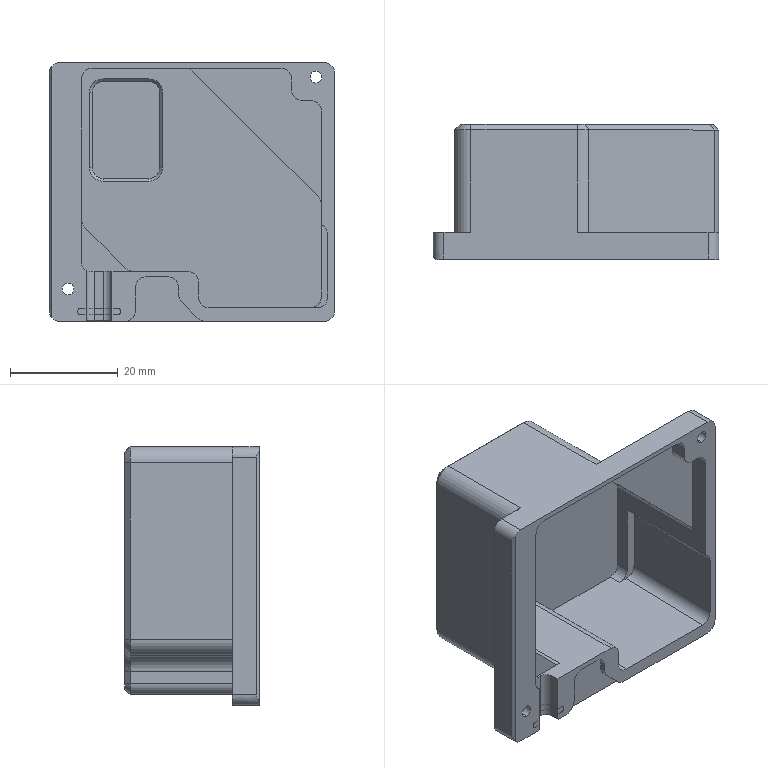NC program | NX | posted with a generic post | part box 53 x 25 x 48 mm
Lines 3425 to 5522 of 6007, first 1921 of 2086 lines:
(CAVITY_MILL_1 , TOOL : D2-6-D4-50-3T-ROUGH)
N6818 T10 M6
N6820 G54
N6822 G17 G0 G90 X25.999 Y-16.249 B0. C0. S6500 M3
N6824 G43 Z30. H10
N6826 Z3.003 B-180. C-180.
N6828 G94 G1 Z0.003 F1200.
N6830 X25.099
N6832 G3 X24.099 Y-17.25 R1.
N6834 G1 Y-18.252
N6836 X24.345 Y-18.329
N6838 X24.41 Y-18.357
N6840 X24.457 Y-18.38
N6842 X24.5 Y-18.406
N6844 X24.821 Y-18.648
N6846 X24.856 Y-18.684
N6848 X24.903 Y-18.731
N6850 X24.955 Y-18.782
N6852 X24.875 Y-19.036
N6854 X24.85 Y-19.062
N6856 X24.842 Y-19.066
N6858 X24.753 Y-18.976
N6860 X24.705 Y-18.929
N6862 X24.649 Y-18.872
N6864 X24.646 Y-18.87
N6866 X24.623 Y-18.846
N6868 X24.333 Y-18.631
N6870 X24.237 Y-18.587
N6872 X24.027 Y-18.523
N6874 X23.912 Y-18.512
N6876 Y-18.5
N6878 X14.606
N6880 X14.555 Y-18.501
N6882 X14.548 Y-18.485
N6884 X14.549 Y-18.452
N6886 X14.585 Y-18.399
N6888 X14.613 Y-18.332
N6890 X14.634 Y-18.271
N6892 X14.689 Y-17.936
N6894 X14.695 Y-16.518
N6896 X14.729 Y-16.405
N6898 X14.772 Y-16.258
N6900 X14.757 Y-16.237
N6902 X14.723 Y-16.214
N6904 X14.701 Y-16.181
N6906 X14.661 Y-16.163
N6908 X14.692 Y-16.132
N6910 X14.727 Y-16.001
N6912 X14.789 Y-16.
N6914 X15.346
N6916 X23.797 Y-15.999
N6918 X24.058 Y-15.971
N6920 G3 X24.602 Y-15.675 R0.932
N6922 G1 X24.797 Y-15.48
N6924 X24.807 Y-15.469
N6926 X24.849 Y-15.429
N6928 X24.894 Y-15.431
N6930 X24.879 Y-15.473
N6932 X24.954 Y-15.718
N6934 X24.805 Y-15.868
N6936 G2 X24.099 Y-16.248 R1.212
N6938 G1 Y-17.25
N6940 X23.199
N6942 Y-17.6
N6944 X15.589
N6946 X15.59 Y-16.9
N6948 X23.199 Y-16.899
N6950 Y-17.25
N6952 G3 X24.199 Y-18.25 R1.
N6954 G1 X25.999 Y-18.249
N6956 Z3.003
N6958 G0 Y-16.25 Z2.855
N6960 G1 Z-0.145
N6962 X25.099
N6964 G3 X24.099 Y-17.25 R1.
N6966 G1 Y-18.252
N6968 G2 X24.463 Y-18.383 R1.43
N6970 X24.841 Y-18.668 R1.431
N6972 G1 X24.903 Y-18.731
N6974 X24.955 Y-18.782
N6976 X24.875 Y-19.036
N6978 X24.842 Y-19.066
N6980 X24.753 Y-18.976
N6982 X24.613 Y-18.837
N6984 G3 X23.912 Y-18.505 R1.15
N6986 G1 Y-18.5
N6988 X23.8
N6990 X14.554 Y-18.501
N6992 X14.548 Y-18.486
N6994 X14.549 Y-18.451
N6996 X14.585 Y-18.399
N6998 X14.613 Y-18.332
N7000 X14.634 Y-18.271
N7002 X14.689 Y-17.936
N7004 X14.695 Y-16.518
N7006 X14.729 Y-16.405
N7008 X14.773 Y-16.259
N7010 X14.757 Y-16.237
N7012 X14.723 Y-16.214
N7014 X14.701 Y-16.181
N7016 X14.661 Y-16.163
N7018 X14.692 Y-16.132
N7020 X14.727 Y-16.001
N7022 X14.788 Y-16.
N7024 X23.8
N7026 G3 X24.058 Y-15.971 R1.15
N7028 X24.613 Y-15.663 R0.933
N7030 G1 X24.808 Y-15.469
N7032 X24.849 Y-15.429
N7034 X24.869 Y-15.449
N7036 X24.888 Y-15.507
N7038 X24.954 Y-15.718
N7040 X24.805 Y-15.868
N7042 G2 X24.099 Y-16.248 R1.213
N7044 G1 Y-17.25
N7046 X23.199
N7048 Y-17.6
N7050 X15.589
N7052 X15.59 Y-16.9
N7054 X23.199
N7056 Y-17.25
N7058 G3 X24.199 Y-18.25 R1.
N7060 G1 X25.999
N7062 Z2.855
N7064 G0 Y-16.25 Z2.708
N7066 G1 Z-0.293
N7068 X25.099
N7070 G3 X24.099 Y-17.25 R1.
N7072 G1 Y-18.252
N7074 G2 X24.841 Y-18.668 R1.431
N7076 G1 X24.903 Y-18.731
N7078 X24.955 Y-18.782
N7080 X24.875 Y-19.036
N7082 X24.842 Y-19.066
N7084 X24.753 Y-18.976
N7086 X24.613 Y-18.837
N7088 G3 X23.912 Y-18.505 R1.15
N7090 G1 Y-18.5
N7092 X23.8
N7094 X14.554 Y-18.501
N7096 X14.548 Y-18.486
N7098 X14.549 Y-18.451
N7100 X14.585 Y-18.399
N7102 X14.613 Y-18.332
N7104 X14.634 Y-18.271
N7106 X14.689 Y-17.936
N7108 X14.695 Y-16.518
N7110 X14.729 Y-16.405
N7112 X14.773 Y-16.259
N7114 X14.757 Y-16.237
N7116 X14.723 Y-16.214
N7118 X14.701 Y-16.181
N7120 X14.661 Y-16.163
N7122 X14.692 Y-16.132
N7124 X14.727 Y-16.001
N7126 X14.788 Y-16.
N7128 X23.8
N7130 G3 X24.058 Y-15.971 R1.15
N7132 G1 X24.188 Y-15.94
N7134 G3 X24.613 Y-15.663 R0.933
N7136 G1 X24.808 Y-15.469
N7138 X24.849 Y-15.429
N7140 X24.869 Y-15.449
N7142 X24.888 Y-15.507
N7144 X24.954 Y-15.718
N7146 X24.805 Y-15.868
N7148 G2 X24.099 Y-16.248 R1.213
N7150 G1 Y-17.25
N7152 X23.199
N7154 Y-17.6
N7156 X15.589
N7158 X15.59 Y-16.9
N7160 X23.199
N7162 Y-17.25
N7164 G3 X24.199 Y-18.25 R1.
N7166 G1 X25.999
N7168 Z2.708
N7170 G0 Y-16.25 Z2.56
N7172 G1 Z-0.44
N7174 X25.099
N7176 G3 X24.099 Y-17.25 R1.
N7178 G1 Y-18.252
N7180 G2 X24.811 Y-18.639 R1.43
N7182 G1 X24.955 Y-18.782
N7184 X24.875 Y-19.036
N7186 X24.842 Y-19.066
N7188 X24.753 Y-18.976
N7190 X24.613 Y-18.837
N7192 G3 X23.912 Y-18.505 R1.15
N7194 G1 Y-18.5
N7196 X23.8
N7198 X14.554 Y-18.501
N7200 X14.548 Y-18.486
N7202 X14.549 Y-18.452
N7204 X14.585 Y-18.399
N7206 X14.613 Y-18.332
N7208 X14.634 Y-18.271
N7210 X14.689 Y-17.936
N7212 X14.695 Y-16.518
N7214 X14.729 Y-16.405
N7216 X14.773 Y-16.259
N7218 X14.757 Y-16.237
N7220 X14.723 Y-16.214
N7222 X14.701 Y-16.181
N7224 X14.661 Y-16.163
N7226 X14.692 Y-16.132
N7228 X14.727 Y-16.001
N7230 X14.788 Y-16.
N7232 X23.8
N7234 G3 X24.058 Y-15.971 R1.15
N7236 X24.376 Y-15.858 R0.932
N7238 X24.613 Y-15.663 R0.933
N7240 G1 X24.808 Y-15.469
N7242 X24.849 Y-15.429
N7244 X24.869 Y-15.449
N7246 X24.888 Y-15.507
N7248 X24.954 Y-15.718
N7250 X24.805 Y-15.868
N7252 G2 X24.099 Y-16.248 R1.213
N7254 G1 Y-17.25
N7256 X23.199
N7258 Y-17.6
N7260 X15.589
N7262 X15.59 Y-16.9
N7264 X23.199
N7266 Y-17.25
N7268 G3 X24.199 Y-18.25 R1.
N7270 G1 X25.999
N7272 Z2.56
N7274 G0 Y-16.25 Z2.413
N7276 G1 Z-0.588
N7278 X25.099
N7280 G3 X24.099 Y-17.25 R1.
N7282 G1 Y-18.252
N7284 G2 X24.811 Y-18.639 R1.43
N7286 G1 X24.955 Y-18.782
N7288 X24.875 Y-19.036
N7290 X24.842 Y-19.066
N7292 X24.753 Y-18.976
N7294 X24.613 Y-18.837
N7296 G3 X23.912 Y-18.505 R1.15
N7298 G1 Y-18.5
N7300 X23.8
N7302 X14.554 Y-18.501
N7304 X14.548 Y-18.486
N7306 X14.549 Y-18.452
N7308 X14.585 Y-18.399
N7310 X14.613 Y-18.332
N7312 X14.634 Y-18.271
N7314 X14.689 Y-17.936
N7316 X14.695 Y-16.518
N7318 X14.729 Y-16.405
N7320 X14.773 Y-16.259
N7322 X14.757 Y-16.237
N7324 X14.723 Y-16.214
N7326 X14.701 Y-16.181
N7328 X14.661 Y-16.163
N7330 X14.692 Y-16.132
N7332 X14.727 Y-16.001
N7334 X14.788 Y-16.
N7336 X23.8
N7338 G3 X24.058 Y-15.971 R1.15
N7340 X24.613 Y-15.663 R0.933
N7342 G1 X24.849 Y-15.429
N7344 X24.869 Y-15.449
N7346 X24.888 Y-15.507
N7348 X24.954 Y-15.718
N7350 X24.805 Y-15.868
N7352 G2 X24.099 Y-16.248 R1.213
N7354 G1 Y-17.25
N7356 X23.199
N7358 Y-17.6
N7360 X15.589
N7362 X15.59 Y-16.9
N7364 X23.199
N7366 Y-17.25
N7368 G3 X24.199 Y-18.25 R1.
N7370 G1 X25.999
N7372 Z2.413
N7374 G0 Y-16.25 Z2.265
N7376 G1 Z-0.735
N7378 X25.099
N7380 G3 X24.099 Y-17.25 R1.
N7382 G1 Y-18.252
N7384 G2 X24.811 Y-18.639 R1.43
N7386 G1 X24.955 Y-18.782
N7388 X24.875 Y-19.036
N7390 X24.842 Y-19.066
N7392 X24.753 Y-18.976
N7394 X24.613 Y-18.837
N7396 G3 X23.912 Y-18.505 R1.15
N7398 G1 Y-18.5
N7400 X23.8
N7402 X14.554 Y-18.501
N7404 X14.548 Y-18.485
N7406 X14.549 Y-18.452
N7408 X14.585 Y-18.399
N7410 X14.613 Y-18.332
N7412 X14.634 Y-18.271
N7414 X14.689 Y-17.936
N7416 X14.695 Y-16.518
N7418 X14.729 Y-16.405
N7420 X14.772 Y-16.258
N7422 X14.757 Y-16.237
N7424 X14.723 Y-16.214
N7426 X14.701 Y-16.181
N7428 X14.661 Y-16.163
N7430 X14.692 Y-16.132
N7432 X14.727 Y-16.001
N7434 X14.788 Y-16.
N7436 X23.8
N7438 G3 X24.058 Y-15.971 R1.15
N7440 X24.613 Y-15.663 R0.933
N7442 G1 X24.808 Y-15.469
N7444 X24.849 Y-15.429
N7446 X24.869 Y-15.449
N7448 X24.888 Y-15.507
N7450 X24.954 Y-15.718
N7452 X24.805 Y-15.868
N7454 G2 X24.099 Y-16.248 R1.213
N7456 G1 Y-17.25
N7458 X23.199
N7460 Y-17.6
N7462 X15.589
N7464 X15.59 Y-16.9
N7466 X23.199
N7468 Y-17.25
N7470 G3 X24.199 Y-18.25 R1.
N7472 G1 X25.999
N7474 Z2.265
N7476 G0 Y-16.25 Z2.118
N7478 G1 Z-0.883
N7480 X25.099
N7482 G3 X24.099 Y-17.25 R1.
N7484 G1 Y-18.252
N7486 G2 X24.811 Y-18.639 R1.43
N7488 G1 X24.955 Y-18.782
N7490 X24.875 Y-19.036
N7492 X24.842 Y-19.066
N7494 X24.753 Y-18.976
N7496 X24.613 Y-18.837
N7498 G3 X23.912 Y-18.505 R1.15
N7500 G1 Y-18.5
N7502 X23.8
N7504 X14.554 Y-18.501
N7506 X14.548 Y-18.485
N7508 X14.549 Y-18.452
N7510 X14.585 Y-18.399
N7512 X14.613 Y-18.332
N7514 X14.634 Y-18.271
N7516 X14.689 Y-17.936
N7518 X14.695 Y-16.518
N7520 X14.729 Y-16.405
N7522 X14.773 Y-16.259
N7524 X14.757 Y-16.237
N7526 X14.723 Y-16.214
N7528 X14.701 Y-16.181
N7530 X14.661 Y-16.163
N7532 X14.692 Y-16.132
N7534 X14.727 Y-16.001
N7536 X14.788 Y-16.
N7538 X23.8
N7540 G3 X24.058 Y-15.971 R1.15
N7542 X24.613 Y-15.663 R0.933
N7544 G1 X24.808 Y-15.469
N7546 X24.849 Y-15.429
N7548 X24.869 Y-15.449
N7550 X24.888 Y-15.507
N7552 X24.954 Y-15.718
N7554 X24.805 Y-15.868
N7556 G2 X24.099 Y-16.248 R1.213
N7558 G1 Y-17.25
N7560 X23.199
N7562 Y-17.6
N7564 X15.589
N7566 X15.59 Y-16.9
N7568 X23.199
N7570 Y-17.25
N7572 G3 X24.199 Y-18.25 R1.
N7574 G1 X25.999
N7576 Z2.118
N7578 G0 Y-16.25 Z1.97
N7580 G1 Z-1.03
N7582 X25.099
N7584 G3 X24.099 Y-17.25 R1.
N7586 G1 Y-18.252
N7588 G2 X24.811 Y-18.639 R1.43
N7590 G1 X24.955 Y-18.782
N7592 X24.875 Y-19.036
N7594 X24.842 Y-19.066
N7596 X24.753 Y-18.976
N7598 X24.613 Y-18.837
N7600 G3 X23.912 Y-18.505 R1.15
N7602 G1 Y-18.5
N7604 X23.8
N7606 X14.554 Y-18.501
N7608 X14.548 Y-18.485
N7610 X14.549 Y-18.453
N7612 X14.585 Y-18.399
N7614 X14.613 Y-18.332
N7616 X14.634 Y-18.271
N7618 X14.689 Y-17.936
N7620 X14.695 Y-16.518
N7622 X14.729 Y-16.405
N7624 X14.773 Y-16.259
N7626 X14.757 Y-16.237
N7628 X14.723 Y-16.214
N7630 X14.701 Y-16.181
N7632 X14.661 Y-16.163
N7634 X14.692 Y-16.132
N7636 X14.727 Y-16.001
N7638 X14.788 Y-16.
N7640 X23.8
N7642 G3 X24.058 Y-15.971 R1.15
N7644 X24.613 Y-15.663 R0.933
N7646 G1 X24.808 Y-15.469
N7648 X24.849 Y-15.429
N7650 X24.869 Y-15.449
N7652 X24.888 Y-15.507
N7654 X24.954 Y-15.718
N7656 X24.805 Y-15.868
N7658 G2 X24.099 Y-16.248 R1.213
N7660 G1 Y-17.25
N7662 X23.199
N7664 Y-17.6
N7666 X15.589
N7668 X15.59 Y-16.9
N7670 X23.199
N7672 Y-17.25
N7674 G3 X24.199 Y-18.25 R1.
N7676 G1 X25.999
N7678 Z1.97
N7680 G0 Y-16.25 Z1.823
N7682 G1 Z-1.178
N7684 X25.099
N7686 G3 X24.099 Y-17.25 R1.
N7688 G1 Y-18.252
N7690 G2 X24.811 Y-18.639 R1.43
N7692 G1 X24.955 Y-18.782
N7694 X24.875 Y-19.036
N7696 X24.842 Y-19.066
N7698 X24.753 Y-18.976
N7700 X24.613 Y-18.837
N7702 G3 X23.912 Y-18.505 R1.15
N7704 G1 Y-18.5
N7706 X23.8
N7708 X14.554 Y-18.501
N7710 X14.548 Y-18.484
N7712 X14.549 Y-18.453
N7714 X14.585 Y-18.399
N7716 X14.613 Y-18.332
N7718 X14.634 Y-18.271
N7720 X14.689 Y-17.936
N7722 X14.695 Y-16.518
N7724 X14.729 Y-16.405
N7726 X14.773 Y-16.259
N7728 X14.757 Y-16.237
N7730 X14.723 Y-16.214
N7732 X14.701 Y-16.181
N7734 X14.661 Y-16.163
N7736 X14.692 Y-16.132
N7738 X14.727 Y-16.001
N7740 X14.735 Y-16.
N7742 X14.788
N7744 X23.8
N7746 G3 X24.058 Y-15.971 R1.15
N7748 X24.613 Y-15.663 R0.933
N7750 G1 X24.849 Y-15.429
N7752 X24.869 Y-15.449
N7754 X24.888 Y-15.507
N7756 X24.954 Y-15.718
N7758 X24.805 Y-15.868
N7760 G2 X24.099 Y-16.248 R1.213
N7762 G1 Y-17.25
N7764 X23.199
N7766 Y-17.6
N7768 X15.589
N7770 X15.59 Y-16.9
N7772 X23.199
N7774 Y-17.25
N7776 G3 X24.199 Y-18.25 R1.
N7778 G1 X25.999
N7780 Z1.823
N7782 G0 Y-16.25 Z1.675
N7784 G1 Z-1.325
N7786 X25.099
N7788 G3 X24.099 Y-17.25 R1.
N7790 G1 Y-18.252
N7792 G2 X24.811 Y-18.639 R1.43
N7794 G1 X24.955 Y-18.782
N7796 X24.875 Y-19.036
N7798 X24.842 Y-19.066
N7800 X24.753 Y-18.976
N7802 X24.613 Y-18.837
N7804 G3 X23.912 Y-18.505 R1.15
N7806 G1 Y-18.5
N7808 X23.8
N7810 X14.554 Y-18.501
N7812 X14.548 Y-18.484
N7814 X14.549 Y-18.453
N7816 X14.585 Y-18.399
N7818 X14.613 Y-18.332
N7820 X14.634 Y-18.271
N7822 X14.689 Y-17.936
N7824 X14.695 Y-16.518
N7826 X14.729 Y-16.405
N7828 X14.773 Y-16.259
N7830 X14.757 Y-16.237
N7832 X14.723 Y-16.214
N7834 X14.701 Y-16.181
N7836 X14.661 Y-16.163
N7838 X14.692 Y-16.132
N7840 X14.727 Y-16.001
N7842 X14.788 Y-16.
N7844 X23.8
N7846 G3 X24.058 Y-15.971 R1.15
N7848 G1 X24.236 Y-15.923
N7850 G3 X24.613 Y-15.663 R0.933
N7852 G1 X24.808 Y-15.469
N7854 X24.849 Y-15.429
N7856 X24.869 Y-15.449
N7858 X24.888 Y-15.507
N7860 X24.954 Y-15.718
N7862 X24.805 Y-15.868
N7864 G2 X24.099 Y-16.248 R1.213
N7866 G1 Y-17.25
N7868 X23.199
N7870 Y-17.6
N7872 X15.589
N7874 X15.59 Y-16.9
N7876 X23.199
N7878 Y-17.25
N7880 G3 X24.199 Y-18.25 R1.
N7882 G1 X25.999
N7884 Z1.675
N7886 G0 Y-16.25 Z1.528
N7888 G1 Z-1.473
N7890 X25.099
N7892 G3 X24.099 Y-17.25 R1.
N7894 G1 Y-18.252
N7896 G2 X24.834 Y-18.661 R1.43
N7898 G1 X24.955 Y-18.782
N7900 X24.876 Y-19.035
N7902 X24.843 Y-19.065
N7904 X24.805 Y-19.027
N7906 X24.753 Y-18.976
N7908 X24.613 Y-18.837
N7910 G3 X23.912 Y-18.505 R1.15
N7912 G1 Y-18.5
N7914 X23.797
N7916 X14.554 Y-18.501
N7918 X14.548 Y-18.484
N7920 X14.549 Y-18.454
N7922 X14.585 Y-18.399
N7924 X14.613 Y-18.332
N7926 X14.634 Y-18.271
N7928 X14.689 Y-17.936
N7930 X14.695 Y-16.518
N7932 X14.729 Y-16.405
N7934 X14.773 Y-16.259
N7936 X14.757 Y-16.237
N7938 X14.723 Y-16.214
N7940 X14.701 Y-16.181
N7942 X14.661 Y-16.163
N7944 X14.692 Y-16.132
N7946 X14.726 Y-16.004
N7948 X14.833 Y-16.
N7950 X23.8
N7952 G3 X24.058 Y-15.971 R1.15
N7954 X24.613 Y-15.663 R0.933
N7956 G1 X24.808 Y-15.469
N7958 X24.849 Y-15.429
N7960 X24.869 Y-15.449
N7962 X24.888 Y-15.507
N7964 X24.954 Y-15.718
N7966 X24.805 Y-15.868
N7968 G2 X24.099 Y-16.248 R1.213
N7970 G1 Y-17.25
N7972 X23.199
N7974 Y-17.6
N7976 X15.589
N7978 X15.59 Y-16.9
N7980 X23.199
N7982 Y-17.25
N7984 G3 X24.199 Y-18.25 R1.
N7986 G1 X25.999
N7988 Z1.528
N7990 G0 Y-16.25 Z1.38
N7992 G1 Z-1.62
N7994 X25.099
N7996 G3 X24.099 Y-17.25 R1.
N7998 G1 Y-18.238
N8000 G2 X24.963 Y-18.758 R1.488
N8002 G1 X24.941 Y-18.82
N8004 X24.879 Y-19.026
N8006 X24.87 Y-19.045
N8008 X24.85 Y-19.062
N8010 X24.807 Y-19.016
N8012 G3 X23.8 Y-18.489 R1.208
N8014 G1 X14.606
N8016 X14.549
N8018 X14.548 Y-18.484
N8020 Y-18.454
N8022 X14.585 Y-18.399
N8024 X14.613 Y-18.332
N8026 X14.634 Y-18.271
N8028 X14.689 Y-17.936
N8030 X14.695 Y-16.518
N8032 X14.729 Y-16.405
N8034 X14.773 Y-16.259
N8036 X14.757 Y-16.237
N8038 X14.723 Y-16.214
N8040 X14.701 Y-16.181
N8042 X14.661 Y-16.163
N8044 X14.692 Y-16.132
N8046 X14.724 Y-16.013
N8048 X15.59 Y-16.011
N8050 X23.88
N8052 G3 X24.331 Y-15.893 R0.924
N8054 X24.818 Y-15.473 R1.602
N8056 G1 X24.855 Y-15.433
N8058 X24.861 Y-15.439
N8060 X24.879 Y-15.473
N8062 X24.94 Y-15.68
N8064 X24.962 Y-15.738
N8066 G2 X24.468 Y-16.138 R1.882
N8068 X24.099 Y-16.271 R1.204
N8070 G1 Y-17.25
N8072 X23.199
N8074 Y-17.589
N8076 X15.589
N8078 X15.59 Y-16.911
N8080 X23.199
N8082 Y-17.25
N8084 G3 X24.199 Y-18.25 R1.
N8086 G1 X25.999
N8088 Z1.38
N8090 G0 Y-16.25 Z1.233
N8092 G1 Z-1.768
N8094 X25.099
N8096 G3 X24.099 Y-17.25 R1.
N8098 G1 Y-18.211
N8100 G2 X24.97 Y-18.739 R1.495
N8102 G1 X24.941 Y-18.82
N8104 X24.879 Y-19.026
N8106 X24.864 Y-19.052
N8108 X24.821 Y-19.009
N8110 G3 X23.8 Y-18.462 R1.215
N8112 G1 X14.621
N8114 X14.547
N8116 X14.558 Y-18.434
N8118 X14.585 Y-18.399
N8120 X14.613 Y-18.332
N8122 X14.634 Y-18.271
N8124 X14.689 Y-17.936
N8126 X14.695 Y-16.518
N8128 X14.729 Y-16.405
N8130 X14.772 Y-16.258
N8132 X14.757 Y-16.237
N8134 X14.723 Y-16.214
N8136 X14.701 Y-16.181
N8138 X14.661 Y-16.163
N8140 X14.692 Y-16.132
N8142 X14.717 Y-16.039
N8144 X15.59 Y-16.038
N8146 X23.8
N8148 G3 X24.839 Y-15.473 R1.25
N8150 G1 X24.866 Y-15.444
N8152 X24.888 Y-15.507
N8154 X24.94 Y-15.68
N8156 X24.971 Y-15.765
N8158 G2 X24.099 Y-16.287 R1.53
N8160 G1 Y-17.25
N8162 X23.199
N8164 Y-17.562
N8166 X15.589
N8168 X15.59 Y-16.938
N8170 X23.199
N8172 Y-17.25
N8174 G3 X24.199 Y-18.25 R1.
N8176 G1 X25.999
N8178 Z1.233
N8180 G0 Y-16.25 Z1.085
N8182 G1 Z-1.915
N8184 X25.099
N8186 G3 X24.099 Y-17.25 R1.
N8188 G1 Y-18.162
N8190 G2 X24.891 Y-18.625 R1.379
N8192 G1 X24.976 Y-18.723
N8194 X24.941 Y-18.82
N8196 X24.877 Y-19.032
N8198 X24.829 Y-18.982
N8200 X24.678 Y-18.807
N8202 G3 X23.8 Y-18.417 R1.099
N8204 G1 X14.642
N8206 X14.569 Y-18.42
N8208 X14.585 Y-18.399
N8210 X14.613 Y-18.332
N8212 X14.634 Y-18.271
N8214 X14.689 Y-17.936
N8216 X14.695 Y-16.518
N8218 X14.729 Y-16.405
N8220 X14.771 Y-16.258
N8222 X14.757 Y-16.237
N8224 X14.723 Y-16.214
N8226 X14.701 Y-16.181
N8228 X14.661 Y-16.163
N8230 X14.692 Y-16.132
N8232 X14.705 Y-16.082
N8234 X15.59 Y-16.083
N8236 X23.8
N8238 G3 X24.84 Y-15.512 R1.298
N8240 G1 X24.878 Y-15.469
N8242 X24.94 Y-15.68
N8244 X24.981 Y-15.79
N8246 G2 X24.099 Y-16.327 R1.578
N8248 G1 Y-17.25
N8250 X23.199
N8252 Y-17.517
N8254 X15.589
N8256 X15.59 Y-16.983
N8258 X23.199
N8260 Y-17.25
N8262 G3 X24.199 Y-18.25 R1.
N8264 G1 X25.999
N8266 Z1.085
N8268 G0 Y-16.25 Z0.938
N8270 G1 Z-2.063
N8272 X25.099
N8274 G3 X24.099 Y-17.25 R1.
N8276 G1 Y-18.092
N8278 G2 X24.781 Y-18.458 R1.238
N8280 G1 X24.992 Y-18.68
N8282 X24.941 Y-18.82
N8284 X24.891 Y-18.984
N8286 X24.85 Y-18.937
N8288 X24.578 Y-18.651
N8290 G3 X23.884 Y-18.353 R0.958
N8292 G1 X14.603 Y-18.355
N8294 X14.634 Y-18.271
N8296 X14.689 Y-17.936
N8298 X14.695 Y-16.518
N8300 X14.729 Y-16.405
N8302 X14.773 Y-16.259
N8304 X14.757 Y-16.237
N8306 X14.723 Y-16.214
N8308 X14.701 Y-16.181
N8310 X14.69 Y-16.147
N8312 X14.75
N8314 X23.854
N8316 G3 X24.559 Y-15.857 R1.
N8318 G1 X24.843 Y-15.575
N8320 X24.891 Y-15.516
N8322 X24.94 Y-15.68
N8324 X24.992 Y-15.821
N8326 X24.756 Y-16.056
N8328 G2 X24.099 Y-16.403 R1.28
N8330 G1 Y-17.25
N8332 X23.199
N8334 Y-17.453
N8336 X15.589
N8338 X15.59 Y-17.047
N8340 X23.199
N8342 Y-17.25
N8344 G3 X24.199 Y-18.25 R1.
N8346 G1 X25.999
N8348 Z0.938
N8350 G0 Y-16.25 Z0.79
N8352 G1 Z-2.21
N8354 X25.099
N8356 G3 X24.099 Y-17.25 R1.
N8358 G1 Y-18.007
N8360 G2 X24.814 Y-18.402 R1.293
N8362 G1 X24.945 Y-18.542
N8364 X24.999 Y-18.6
N8366 Y-18.659
N8368 X24.941 Y-18.82
N8370 X24.906 Y-18.935
N8372 X24.817 Y-18.822
N8374 X24.766 Y-18.756
N8376 X24.74 Y-18.735
N8378 X24.609 Y-18.592
N8380 G3 X23.864 Y-18.266 R1.013
N8382 G1 X14.698
N8384 X14.635 Y-18.268
N8386 X14.689 Y-17.936
N8388 X14.695 Y-16.518
N8390 X14.729 Y-16.405
N8392 X14.773 Y-16.259
N8394 X14.757 Y-16.237
N8396 X14.749 Y-16.234
N8398 X15.59
N8400 X23.8
N8402 G3 X24.852 Y-15.634 R1.342
N8404 G1 X24.906 Y-15.566
N8406 X24.94 Y-15.68
N8408 X24.999 Y-15.841
N8410 Y-15.907
N8412 G2 X24.099 Y-16.474 R1.622
N8414 G1 Y-17.25
N8416 X23.199
N8418 Y-17.366
N8420 X15.589
N8422 X15.59 Y-17.134
N8424 X23.199
N8426 Y-17.25
N8428 G3 X24.199 Y-18.25 R1.
N8430 G1 X25.999
N8432 Z0.79
N8434 G0 Y-16.239 Z0.643
N8436 G1 Z-2.358
N8438 X25.099
N8440 G3 X24.099 Y-17.239 R1.
N8442 G1 Y-17.889
N8444 G2 X24.909 Y-18.392 R1.276
N8446 G1 X24.999 Y-18.515
N8448 Y-18.659
N8450 X24.922 Y-18.881
N8452 X24.683 Y-18.558
N8454 G3 X23.88 Y-18.149 R0.996
N8456 G1 X14.726
N8458 X14.654 Y-18.153
N8460 X14.689 Y-17.936
N8462 X14.695 Y-16.518
N8464 X14.729 Y-16.405
N8466 X14.745 Y-16.351
N8468 X23.8
N8470 G3 X24.865 Y-15.699 R1.317
N8472 G1 X24.924 Y-15.625
N8474 X24.94 Y-15.68
N8476 X24.999 Y-15.841
N8478 Y-16.002
N8480 G2 X24.099 Y-16.589 R1.597
N8482 G1 Y-17.239
N8484 G3 X25.099 Y-18.239 R1.
N8486 G1 X25.999
N8488 Z0.643
N8490 G0 Y-16.238 Z0.495
N8492 G1 Z-2.505
N8494 X25.099
N8496 G3 X24.099 Y-17.238 R1.
N8498 G1 Y-17.722
N8500 G2 X24.62 Y-17.956 R1.019
N8502 X24.999 Y-18.363 R2.447
N8504 G1 Y-18.659
N8506 X24.947 Y-18.803
N8508 G3 X24.438 Y-18.169 R2.167
N8510 X23.959 Y-17.992 R0.739
N8512 G1 X14.746
N8514 X14.679 Y-17.996
N8516 X14.689 Y-17.936
N8518 X14.696 Y-16.515
N8520 X14.75 Y-16.508
N8522 X23.8
N8524 G3 X24.894 Y-15.776 R1.205
N8526 G1 X24.946 Y-15.696
N8528 X24.999 Y-15.841
N8530 Y-16.159
N8532 G2 X24.099 Y-16.754 R1.485
N8534 G1 Y-17.238
N8536 G3 X25.099 Y-18.238 R1.
N8538 G1 X25.999
N8540 Z0.495
N8542 G0 Y-17.384 Z0.348
N8544 G1 Z-2.653
N8546 G3 X24.999 Y-18.384 R1.
N8548 G1 Y-18.659
N8550 X24.977 Y-18.722
N8552 X24.692 Y-18.19
N8554 G3 X23.979 Y-17.764 R0.809
N8556 G1 X14.75
N8558 X14.689 Y-17.758
N8560 X14.69 Y-16.741
N8562 X14.75 Y-16.736
N8564 X23.8
N8566 G3 X24.948 Y-15.866 R1.325
N8568 G1 X24.985 Y-15.803
N8570 X24.999 Y-15.841
N8572 Y-16.36
N8574 G2 X24.099 Y-16.97 R1.605
N8576 G1 Y-17.49
N8578 G2 X24.939 Y-18.058 R1.089
N8580 G1 X24.999 Y-18.171
N8582 Y-18.384
N8584 G3 X25.999 Y-19.384 R1.
N8586 G1 X26.15
N8588 Z0.348
N8590 G0 X12.649 Y-17.258 Z0.2
N8592 G1 Z-2.8
N8594 X14.689 Y-17.259
N8596 Y-17.217
N8598 X14.75 Y-17.208
N8600 X23.8
N8602 X23.797 Y-17.292
N8604 X14.75
N8606 X14.689 Y-17.3
N8608 Y-17.259
N8610 Z0.2
N8612 G0 Z0.348
N8614 X26.147 Y-15.417
N8616 Z0.2
N8618 G1 Z-2.8
N8620 G3 X24.999 Y-15.967 R1.
N8622 G1 X24.982 Y-16.001
N8624 G2 X23.992 Y-17.298 R2.123
N8626 X24.985 Y-18.496 R1.734
N8628 G1 X24.999 Y-18.535
N8630 G3 X26.15 Y-19.184 R1.
N8632 G1 Z0.2
N8634 G0 Y-15.517 Z0.083
N8636 G1 Z-2.917
N8638 G3 X24.999 Y-16.266 R1.
N8640 G1 X24.979 Y-16.35
N8642 Y-18.15
N8644 X24.999 Y-18.231
N8646 G3 X26.15 Y-18.969 R1.
N8648 G1 Z0.083
N8650 G0 Z30.
(PLANAR_MILL_9 , TOOL : D2-6-D4-50-3T-ROUGH)
N8652 X10.25 Y-18.5 S4500
N8654 Z1.529
N8656 G1 Z-0.471 F300.
N8658 G3 X11.25 Y-19.5 R1.
N8660 G1 X13.25
N8662 G3 X13.75 Y-19. R0.5
N8664 G1 Y-17.
N8666 G3 X12.75 Y-16. R1.
N8668 G1 Z1.529
N8670 G0 X10.25 Y-18.5 Z1.057
N8672 G1 Z-0.943
N8674 G3 X11.25 Y-19.5 R1.
N8676 G1 X13.25
N8678 G3 X13.75 Y-19. R0.5
N8680 G1 Y-17.
N8682 G3 X12.75 Y-16. R1.
N8684 G1 Z1.057
N8686 G0 X10.25 Y-18.5 Z0.586
N8688 G1 Z-1.414
N8690 G3 X11.25 Y-19.5 R1.
N8692 G1 X13.25
N8694 G3 X13.75 Y-19. R0.5
N8696 G1 Y-17.
N8698 G3 X12.75 Y-16. R1.
N8700 G1 Z0.586
N8702 G0 X10.25 Y-18.5 Z0.114
N8704 G1 Z-1.886
N8706 G3 X11.25 Y-19.5 R1.
N8708 G1 X13.25
N8710 G3 X13.75 Y-19. R0.5
N8712 G1 Y-17.
N8714 G3 X12.75 Y-16. R1.
N8716 G1 Z0.114
N8718 G0 X10.25 Y-18.5 Z-0.357
N8720 G1 Z-2.357
N8722 G3 X11.25 Y-19.5 R1.
N8724 G1 X13.25
N8726 G3 X13.75 Y-19. R0.5
N8728 G1 Y-17.
N8730 G3 X12.75 Y-16. R1.
N8732 G1 Z-0.357
N8734 G0 X10.25 Y-18.5 Z-0.829
N8736 G1 Z-2.829
N8738 G3 X11.25 Y-19.5 R1.
N8740 G1 X13.25
N8742 G3 X13.75 Y-19. R0.5
N8744 G1 Y-17.
N8746 G3 X12.75 Y-16. R1.
N8748 G1 Z-0.829
N8750 G0 X10.25 Y-18.5 Z-1.3
N8752 G1 Z-3.3
N8754 G3 X11.25 Y-19.5 R1.
N8756 G1 X13.25
N8758 G3 X13.75 Y-19. R0.5
N8760 G1 Y-17.
N8762 G3 X12.75 Y-16. R1.
N8764 G1 Z-1.3
N8766 G0 Z30.
N8768 M5
(AREA_MILL , TOOL : 球刀R0.75-3-D4-50)
N8770 T11 M6
N8772 G54
N8774 G17 G0 G90 X13.863 Y-18.9 B0. C0. S6500 M3
N8776 G43 Z30. H11
N8778 Z2.815 B-180. C-180.
N8780 G94 G1 Z0. F2000.
N8782 X13.964 Z-0.375
N8784 X14.238 Z-0.649
N8786 X14.613 Z-0.75
N8788 X23.799
N8790 X24.088 Y-18.97
N8792 X24.346 Y-19.118
N8794 X24.344 Y-19.133 Z-0.799
N8796 X24.087 Y-18.957
N8798 X23.8 Y-18.9
N8800 X14.608
N8802 X14.607 Z-0.849
N8804 X23.8
N8806 X24.087 Y-18.957
N8808 X24.33 Y-19.12
N8810 X24.349 Y-19.139
N8812 X24.355 Y-19.144 Z-0.898
N8814 X24.33 Y-19.12
N8816 X24.087 Y-18.957
N8818 X23.8 Y-18.9
N8820 X14.607
N8822 Z-0.947
N8824 X23.8
N8826 X24.087 Y-18.957
N8828 X24.33 Y-19.12
N8830 X24.36 Y-19.15
N8832 X24.366 Y-19.155 Z-0.997
N8834 X24.33 Y-19.12
N8836 X24.087 Y-18.957
N8838 X23.8 Y-18.9
N8840 X14.607
N8842 Z-1.046
N8844 X23.8
N8846 X24.087 Y-18.957
N8848 X24.33 Y-19.12
N8850 X24.371 Y-19.16
N8852 X24.377 Y-19.166 Z-1.096
N8854 X24.33 Y-19.12
N8856 X24.087 Y-18.957
N8858 X23.8 Y-18.9
N8860 X14.606
N8862 Z-1.145
N8864 X23.8
N8866 X24.087 Y-18.957
N8868 X24.33 Y-19.12
N8870 X24.382 Y-19.171
N8872 X24.385 Y-19.174 Z-1.195
N8874 X24.33 Y-19.12
N8876 X24.087 Y-18.957
N8878 X23.8 Y-18.9
N8880 X14.606
N8882 Z-1.244
N8884 X23.8
N8886 X24.087 Y-18.957
N8888 X24.33 Y-19.12
N8890 X24.391 Y-19.18
N8892 X24.396 Y-19.185 Z-1.294
N8894 X24.33 Y-19.12
N8896 X24.087 Y-18.957
N8898 X23.8 Y-18.9
N8900 X14.606
N8902 X14.605 Z-1.343
N8904 X23.8
N8906 X24.087 Y-18.957
N8908 X24.33 Y-19.12
N8910 X24.402 Y-19.191
N8912 X24.407 Y-19.197 Z-1.392
N8914 X24.33 Y-19.12
N8916 X24.087 Y-18.957
N8918 X23.8 Y-18.9
N8920 X14.605
N8922 Z-1.442
N8924 X23.8
N8926 X24.087 Y-18.957
N8928 X24.33 Y-19.12
N8930 X24.413 Y-19.202
N8932 X24.418 Y-19.208 Z-1.491
N8934 X24.33 Y-19.12
N8936 X24.087 Y-18.957
N8938 X23.8 Y-18.9
N8940 X14.605
N8942 Z-1.541
N8944 X23.8
N8946 X24.087 Y-18.957
N8948 X24.33 Y-19.12
N8950 X24.427 Y-19.216
N8952 X24.432 Y-19.222 Z-1.59
N8954 X24.33 Y-19.12
N8956 X24.087 Y-18.957
N8958 X23.8 Y-18.9
N8960 X14.604
N8962 Z-1.64
N8964 X23.8
N8966 X24.087 Y-18.957
N8968 X24.33 Y-19.12
N8970 X24.438 Y-19.227
N8972 X24.443 Y-19.232 Z-1.689
N8974 X24.33 Y-19.12
N8976 X24.087 Y-18.957
N8978 X23.8 Y-18.9
N8980 X14.604
N8982 Z-1.738
N8984 X23.8
N8986 X24.087 Y-18.957
N8988 X24.33 Y-19.12
N8990 X24.448 Y-19.238
N8992 X24.454 Y-19.243 Z-1.788
N8994 X24.33 Y-19.12
N8996 X24.087 Y-18.957
N8998 X23.8 Y-18.9
N9000 X14.604
N9002 X14.603 Z-1.837
N9004 X23.8
N9006 X24.087 Y-18.957
N9008 X24.33 Y-19.12
N9010 X24.457 Y-19.246
N9012 X24.462 Y-19.252 Z-1.887
N9014 X24.33 Y-19.12
N9016 X24.087 Y-18.957
N9018 X23.8 Y-18.9
N9020 X14.603
N9022 Z-1.936
N9024 X23.8
N9026 X24.087 Y-18.957
N9028 X24.33 Y-19.12
N9030 X24.468 Y-19.257
N9032 X24.473 Y-19.263 Z-1.986
N9034 X24.33 Y-19.12
N9036 X24.087 Y-18.957
N9038 X23.8 Y-18.9
N9040 X14.603
N9042 Z-2.035
N9044 X23.8
N9046 X24.087 Y-18.957
N9048 X24.33 Y-19.12
N9050 X24.482 Y-19.271
N9052 X24.487 Y-19.277 Z-2.085
N9054 X24.33 Y-19.12
N9056 X24.087 Y-18.957
N9058 X23.8 Y-18.9
N9060 X14.602
N9062 Z-2.134
N9064 X23.8
N9066 X24.087 Y-18.957
N9068 X24.33 Y-19.12
N9070 X24.492 Y-19.282
N9072 X24.495 Y-19.285 Z-2.183
N9074 X24.33 Y-19.12
N9076 X24.123 Y-18.973
N9078 X23.878 Y-18.904
N9080 X23.535 Y-18.9
N9082 X14.602
N9084 X14.601 Z-2.233
N9086 X23.793
N9088 X24.088 Y-18.947
N9090 X24.334 Y-19.116
N9092 X24.517 Y-19.28
N9094 X24.526 Y-19.282 Z-2.282
N9096 X24.339 Y-19.111
N9098 X24.095 Y-18.94
N9100 X23.8 Y-18.895
N9102 X14.606
N9104 X14.608 Y-18.888 Z-2.332
N9106 X23.8
N9108 X24.098 Y-18.933
N9110 X24.344 Y-19.106
N9112 X24.535 Y-19.285
N9114 X24.536 Y-19.289 Z-2.381
N9116 X24.461 Y-19.215
N9118 X24.174 Y-18.962
N9120 X23.8 Y-18.878
N9122 X14.617
N9124 X14.629 Y-18.864 Z-2.431
N9126 X23.8
N9128 X23.87 Y-18.846
N9130 X24.133 Y-18.931
N9132 X24.354 Y-19.096
N9134 X24.554 Y-19.293
N9136 X24.561 Y-19.303 Z-2.48
N9138 X24.345 Y-19.066
N9140 X24.063 Y-18.882
N9142 X23.87 Y-18.821
N9144 X23.8 Y-18.846
N9146 X14.643
N9148 X14.654 Y-18.824 Z-2.529
N9150 X23.8
N9152 X23.87 Y-18.796
N9154 X24.101 Y-18.872
N9156 X24.21 Y-18.946
N9158 X24.405 Y-19.113
N9160 X24.572 Y-19.309
N9162 X24.576 Y-19.303 Z-2.579
N9164 X24.424 Y-19.118
N9166 X24.091 Y-18.836
N9168 X23.87 Y-18.771
N9170 X23.8 Y-18.797
N9172 X14.672
N9174 X14.69 Y-18.766 Z-2.628
N9176 X23.803 Y-18.765
N9178 X23.985 Y-18.761
N9180 X24.148 Y-18.841
N9182 X24.313 Y-18.979
N9184 X24.474 Y-19.136
N9186 X24.575 Y-19.275
N9188 X24.57 Y-19.241 Z-2.678
N9190 X24.471 Y-19.118
N9192 X24.144 Y-18.806
N9194 X23.8 Y-18.728
N9196 X14.708
N9198 X14.724 Y-18.684 Z-2.727
N9200 X23.882 Y-18.683
N9202 X24.06 Y-18.72
N9204 X24.21 Y-18.822
N9206 X24.467 Y-19.087
N9208 X24.562 Y-19.207
N9210 X24.557 Y-19.176 Z-2.777
N9212 X24.466 Y-19.054
N9214 X24.181 Y-18.756
N9216 X24.045 Y-18.662
N9218 X23.882 Y-18.63
N9220 X14.729 Y-18.632
N9222 X14.736 Y-18.566 Z-2.826
N9224 X23.86 Y-18.563
N9226 X24.042 Y-18.602
N9228 X24.192 Y-18.714
N9230 X24.466 Y-19.027
N9232 X24.553 Y-19.143
N9234 X24.551 Y-19.108 Z-2.876
N9236 X24.466 Y-18.987
N9238 X24.145 Y-18.598
N9240 X23.8 Y-18.476
N9242 X14.734 Y-18.474
N9244 X14.74 Y-18.365 Z-2.9
N9246 X14.742 Y-18.343 Z-2.925
N9248 X23.8 Y-18.342
N9250 X24.165 Y-18.544
N9252 X24.41 Y-18.882
N9254 X24.466 Y-18.949
N9256 X24.548 Y-19.068
N9258 X24.761 Y-19.376 Z-2.825
N9260 X24.918 Y-19.602 Z-2.55
N9262 X24.975 Y-19.684 Z-2.175
N9264 Z2.833
N9266 G0 Z30.
N9268 X25.064 Y-14.628
N9270 Z2.811
N9272 G1 Z0.
N9274 X24.994 Y-14.7 Z-0.375
N9276 X24.804 Y-14.898 Z-0.649
N9278 X24.543 Y-15.167 Z-0.75
N9280 X24.307 Y-15.404
N9282 X24.07 Y-15.553
N9284 X23.795 Y-15.6
N9286 X15.033
N9288 X15.022 Z-0.799
N9290 X23.8
N9292 X24.087 Y-15.543
N9294 X24.33 Y-15.38
N9296 X24.544 Y-15.166
N9298 X24.543 Y-15.167 Z-0.849
N9300 X24.33 Y-15.38
N9302 X24.087 Y-15.543
N9304 X23.8 Y-15.6
N9306 X15.012
N9308 X15.002 Z-0.898
N9310 X23.8
N9312 X24.087 Y-15.543
N9314 X24.33 Y-15.38
N9316 X24.542 Y-15.169
N9318 X24.54 Y-15.17 Z-0.947
N9320 X24.33 Y-15.38
N9322 X24.087 Y-15.543
N9324 X23.8 Y-15.6
N9326 X14.992
N9328 X14.983 Z-0.997
N9330 X23.8
N9332 X24.087 Y-15.543
N9334 X24.33 Y-15.38
N9336 X24.539 Y-15.171
N9338 X24.538 Y-15.173 Z-1.046
N9340 X24.33 Y-15.38
N9342 X24.087 Y-15.543
N9344 X23.8 Y-15.6
N9346 X14.973
N9348 X14.963 Z-1.096
N9350 X23.8
N9352 X24.087 Y-15.543
N9354 X24.33 Y-15.38
N9356 X24.537 Y-15.174
N9358 X24.535 Y-15.175 Z-1.145
N9360 X24.33 Y-15.38
N9362 X24.087 Y-15.543
N9364 X23.8 Y-15.6
N9366 X14.956
N9368 X14.946 Z-1.195
N9370 X23.8
N9372 X24.087 Y-15.543
N9374 X24.33 Y-15.38
N9376 X24.534 Y-15.177
N9378 X24.53 Y-15.18 Z-1.244
N9380 X24.33 Y-15.38
N9382 X24.087 Y-15.543
N9384 X23.8 Y-15.6
N9386 X14.93
N9388 X14.921 Z-1.294
N9390 X23.8
N9392 X24.087 Y-15.543
N9394 X24.33 Y-15.38
N9396 X24.529 Y-15.182
N9398 X24.528 Z-1.343
N9400 X24.33 Y-15.38
N9402 X24.087 Y-15.543
N9404 X23.8 Y-15.6
N9406 X14.911
N9408 X14.901 Z-1.392
N9410 X23.8
N9412 X24.087 Y-15.543
N9414 X24.33 Y-15.38
N9416 X24.528 Y-15.183
N9418 X24.527 Y-15.184 Z-1.442
N9420 X24.33 Y-15.38
N9422 X24.087 Y-15.543
N9424 X23.8 Y-15.6
N9426 X14.892
N9428 X14.882 Z-1.491
N9430 X23.8
N9432 X24.087 Y-15.543
N9434 X24.33 Y-15.38
N9436 X24.526 Y-15.184
N9438 Y-15.185 Z-1.541
N9440 X24.33 Y-15.38
N9442 X24.087 Y-15.543
N9444 X23.8 Y-15.6
N9446 X14.872
N9448 X14.862 Z-1.59
N9450 X23.8
N9452 X24.087 Y-15.543
N9454 X24.33 Y-15.38
N9456 X24.522 Y-15.188
N9458 X24.521 Y-15.189 Z-1.64
N9460 X24.33 Y-15.38
N9462 X24.087 Y-15.543
N9464 X23.8 Y-15.6
N9466 X14.853
N9468 X14.84 Z-1.689
N9470 X23.8
N9472 X24.087 Y-15.543
N9474 X24.33 Y-15.38
N9476 X24.52 Y-15.19
N9478 X24.519 Y-15.191 Z-1.738
N9480 X24.33 Y-15.38
N9482 X24.087 Y-15.543
N9484 X23.8 Y-15.6
N9486 X14.831
N9488 X14.821 Z-1.788
N9490 X23.8
N9492 X24.087 Y-15.543
N9494 X24.33 Y-15.38
N9496 X24.518 Y-15.192
N9498 X24.517 Y-15.193 Z-1.837
N9500 X24.33 Y-15.38
N9502 X24.087 Y-15.543
N9504 X23.8 Y-15.6
N9506 X14.812
N9508 X14.802 Z-1.887
N9510 X23.8
N9512 X24.087 Y-15.543
N9514 X24.33 Y-15.38
N9516 X24.514 Y-15.197
N9518 X24.513 Y-15.198 Z-1.936
N9520 X24.33 Y-15.38
N9522 X24.087 Y-15.543
N9524 X23.8 Y-15.6
N9526 X14.79
N9528 X14.781 Z-1.986
N9530 X23.8
N9532 X24.087 Y-15.543
N9534 X24.33 Y-15.38
N9536 X24.512 Y-15.199
N9538 X24.51 Y-15.2 Z-2.035
N9540 X24.33 Y-15.38
N9542 X24.087 Y-15.543
N9544 X23.8 Y-15.6
N9546 X14.776
N9548 X14.762 Z-2.085
N9550 X23.8
N9552 X24.087 Y-15.543
N9554 X24.33 Y-15.38
N9556 X24.509 Y-15.201
N9558 X24.508 Y-15.203 Z-2.134
N9560 X24.33 Y-15.38
N9562 X24.087 Y-15.543
N9564 X23.8 Y-15.6
N9566 X14.75
N9568 Z-2.183
N9570 X23.8
N9572 X24.087 Y-15.543
N9574 X24.33 Y-15.38
N9576 X24.506 Y-15.203
N9578 X24.513 Y-15.214 Z-2.233
N9580 X24.418 Y-15.297
N9582 X24.123 Y-15.531
N9584 X23.752 Y-15.6
N9586 X14.75
N9588 Y-15.605 Z-2.282
N9590 X23.8
N9592 X24.148 Y-15.523
N9594 X24.515 Y-15.218
N9596 X24.517 Y-15.223 Z-2.332
N9598 X24.153 Y-15.527
N9600 X23.8 Y-15.612
N9602 X14.75
N9604 Y-15.622 Z-2.381
N9606 X23.8
N9608 X24.158 Y-15.533
N9610 X24.519 Y-15.228
N9612 X24.52 Y-15.233 Z-2.431
N9614 X24.165 Y-15.543
N9616 X23.8 Y-15.636
N9618 X14.75
N9620 X14.747 Y-15.654 Z-2.48
N9622 X23.8
N9624 X24.144 Y-15.57
N9626 X24.419 Y-15.347
N9628 X24.527 Y-15.247
N9630 X24.52 Y-15.265 Z-2.529
N9632 X24.424 Y-15.352
N9634 X24.307 Y-15.483
N9636 X24.071 Y-15.626
N9638 X23.8 Y-15.676
N9640 X14.75
N9642 X14.747 Y-15.703 Z-2.579
N9644 X23.8
N9646 X24.096 Y-15.648
N9648 X24.336 Y-15.465
N9650 X24.367 Y-15.423
N9652 X24.451 Y-15.355
N9654 X24.52 Y-15.284
N9656 Y-15.304 Z-2.628
N9658 X24.452 Y-15.374
N9660 X24.128 Y-15.66
N9662 X23.8 Y-15.734
N9664 X14.75
N9666 X14.722 Y-15.766
N9668 X14.73 Y-15.803 Z-2.678
N9670 X14.762 Y-15.772
N9672 X23.8
N9674 X24.137 Y-15.686
N9676 X24.454 Y-15.395
N9678 X24.523 Y-15.322
N9680 X24.526 Y-15.345 Z-2.727
N9682 X24.455 Y-15.425
N9684 X24.125 Y-15.731
N9686 X23.8 Y-15.817
N9688 X14.84
N9690 X14.744 Y-15.845
N9692 X14.738 Y-15.911 Z-2.777
N9694 X14.751 Y-15.9
N9696 X14.75 Y-15.87
N9698 X23.8
N9700 X24.136 Y-15.767
N9702 X24.382 Y-15.515
N9704 X24.455 Y-15.448
N9706 X24.528 Y-15.366
N9708 X24.532 Y-15.389 Z-2.826
N9710 X24.456 Y-15.485
N9712 X24.117 Y-15.837
N9714 X23.8 Y-15.937
N9716 X14.75
N9718 X14.759 Y-15.986
N9720 X14.741 Y-16.004
N9722 X14.75 Y-16.024 Z-2.876
N9724 X23.8
N9726 X24.143 Y-15.88
N9728 X24.38 Y-15.595
N9730 X24.457 Y-15.517
N9732 X24.537 Y-15.416
N9734 X24.535 Y-15.456 Z-2.925
N9736 X24.417 Y-15.595
N9738 X24.178 Y-15.916
N9740 X23.889 Y-16.193
N9742 X23.8 Y-16.158
N9744 X14.75
N9746 X14.375 Z-2.825
N9748 X14.1 Z-2.55
N9750 X14. Z-2.175
N9752 Z2.647
N9754 G0 Z30.
N9756 X24.97 Y-19.641
N9758 Z2.832
N9760 G1 Z-2.224
N9762 X24.913 Y-19.558 Z-2.599
N9764 X24.757 Y-19.332 Z-2.874
N9766 X24.544 Y-19.024 Z-2.974
N9768 X24.326 Y-18.717
N9770 X24.202 Y-18.522
N9772 X24.09 Y-18.321
N9774 X23.99 Y-18.113
N9776 Y-16.403
N9778 X23.97 Y-16.345
N9780 X24.518 Y-15.502
N9782 X24.519 Y-15.557 Z-3.024
N9784 X24.459 Y-15.637
N9786 X24.248 Y-16.001
N9788 X24.125 Y-16.403
N9790 Y-18.113
N9792 X24.243 Y-18.499
N9794 X24.547 Y-18.973
N9796 X24.55 Y-18.924 Z-3.073
N9798 X24.466 Y-18.771
N9800 X24.338 Y-18.583
N9802 X24.2 Y-18.155
N9804 X24.212 Y-18.113
N9806 Y-16.381
N9808 X24.345 Y-15.894
N9810 X24.461 Y-15.731
N9812 X24.527 Y-15.619
N9814 X24.528 Y-15.674 Z-3.123
N9816 X24.462 Y-15.792
N9818 X24.397 Y-15.894
N9820 X24.265 Y-16.345
N9822 X24.279 Y-16.381
N9824 Y-18.113
N9826 X24.257 Y-18.155
N9828 X24.39 Y-18.583
N9830 X24.467 Y-18.708
N9832 X24.552 Y-18.872
N9834 X24.557 Y-18.813 Z-3.172
N9836 X24.441 Y-18.583
N9838 X24.333 Y-18.15
N9840 Y-16.35
N9842 X24.448 Y-15.894
N9844 X24.534 Y-15.734
N9846 X24.535 Y-15.786 Z-3.222
N9848 X24.465 Y-15.989
N9850 X24.382 Y-16.35
N9852 Y-18.15
N9854 X24.396 Y-18.284
N9856 X24.554 Y-18.727
N9858 X24.542 Y-18.63 Z-3.271
N9860 X24.463 Y-18.327
N9862 X24.432 Y-18.15
N9864 Y-16.35
N9866 X24.534 Y-15.894
N9868 X24.546 Y-15.867
N9870 X24.572 Y-15.972 Z-3.321
N9872 X24.481 Y-16.35
N9874 Y-18.15
N9876 X24.568 Y-18.506
N9878 X24.543 Y-18.398 Z-3.345
N9880 X24.557 Y-18.281 Z-3.37
N9882 X24.531 Y-18.139
N9884 Y-16.398
N9886 X24.566 Y-16.196
N9888 X24.631 Y-15.827 Z-3.269
N9890 X24.678 Y-15.556 Z-2.995
N9892 X24.695 Y-15.457 Z-2.62
N9894 Z2.812
N9896 G0 Z30.
N9898 X24.869 Y-18.582
N9900 Z2.646
N9902 G1 Z-2.231
N9904 X24.697 Z-2.58
N9906 X24.374 Z-2.795
N9908 X23.987 Z-2.821
N9910 X23.777 Z-2.779
N9912 X18.263 Y-18.583 Z-2.778
N9914 X14.832 Y-18.584 Z-2.785
N9916 X14.75 Z-2.794
N9918 Y-18.545 Z-2.814
N9920 X14.792 Z-2.81
N9922 X23.817 Y-18.543 Z-2.809
N9924 X23.947 Z-2.835
N9926 X24.068 Z-2.87
N9928 X24.09 Y-18.532 Z-2.884
N9930 X24.165 Y-18.503 Z-2.956
N9932 X24.09 Z-2.903
N9934 X23.857 Z-2.84
N9936 X22.806 Z-2.836
N9938 X14.75 Y-18.505 Z-2.835
N9940 Y-18.474 Z-2.853
N9942 X23.413 Y-18.472 Z-2.856
N9944 X23.875 Z-2.861
N9946 X24.09 Z-2.922
N9948 X24.246 Z-3.031
N9950 X24.262 Y-18.465 Z-3.046
N9952 X24.263 Y-18.431 Z-3.055
N9954 X24.09 Z-2.936
N9956 X23.93 Z-2.889
N9958 X23.834 Z-2.875
N9960 X20.526 Y-18.432 Z-2.873
N9962 X14.77 Y-18.434 Z-2.87
N9964 X14.75 Z-2.874
N9966 X14.751 Y-18.391 Z-2.899
N9968 X14.814 Z-2.887
N9970 X23.791 Y-18.388 Z-2.891
N9972 X23.974 Z-2.917
N9974 X24.09 Z-2.951
N9976 X24.207 Z-3.033
N9978 X24.265 Z-3.064
N9980 X24.267 Y-18.345 Z-3.073
N9982 X24.163 Z-3.017
N9984 X24.09 Z-2.966
N9986 X24.017 Z-2.944
N9988 X23.747 Z-2.906
N9990 X14.857 Y-18.348 Z-2.904
N9992 X14.752 Z-2.922
N9994 Y-18.304 Z-2.939
N9996 X14.902 Y-18.303 Z-2.922
N9998 X23.702 Y-18.301 Z-2.921
N10000 X24.062 Z-2.973
N10002 X24.09 Z-2.981
N10004 X24.269 Z-3.082
N10006 X24.271 Y-18.254 Z-3.092
N10008 X24.09 Z-2.994
N10010 X23.674 Z-2.933
N10012 X14.916 Y-18.256 Z-2.936
N10014 X14.751 Z-2.951
N10016 Y-18.207 Z-2.95
N10018 X14.866 Z-2.939
N10020 X23.743 Y-18.205
N10022 X23.951 Z-2.981
N10024 X24.09 Z-3.001
N10026 X24.273 Z-3.101
N10028 X24.27 Y-18.156 Z-3.109
N10030 X24.09 Z-3.007
N10032 X23.793 Z-2.945
N10034 X14.816 Y-18.158 Z-2.943
N10036 X14.751 Z-2.949
N10038 X14.75 Y-18.109
N10040 X23.843 Y-18.106 Z-2.95
N10042 X24.09 Z-3.008
N10044 X24.268 Z-3.116
N10046 Y-18.056 Z-3.12
N10048 X24.09 Z-3.008
N10050 X23.882 Z-2.955
N10052 X22.844 Y-18.057 Z-2.95
N10054 X14.75 Y-18.059
N10056 Y-18.009
N10058 X23.674 Y-18.007
N10060 X23.882 Z-2.955
N10062 X24.09 Y-18.006 Z-3.008
N10064 X24.269 Z-3.121
N10066 X24.27 Y-17.956 Z-3.122
N10068 X24.09 Z-3.008
N10070 X23.882 Y-17.957 Z-2.955
N10072 X22.842 Z-2.95
N10074 X14.75 Y-17.959
N10076 Y-17.909
N10078 X23.674 Y-17.907
N10080 X23.882 Z-2.955
N10082 X24.09 Z-3.008
N10084 X24.272 Y-17.906 Z-3.123
N10086 X24.273 Y-17.856
N10088 X24.09 Y-17.857 Z-3.008
N10090 X23.882 Z-2.955
N10092 X22.845 Z-2.95
N10094 X14.75 Y-17.859
N10096 Y-17.809
N10098 X23.674 Y-17.807
N10100 X23.882 Z-2.955
N10102 X24.09 Z-3.008
N10104 X24.273 Y-17.806 Z-3.123
N10106 X24.272 Y-17.756
N10108 X24.09 Y-17.757 Z-3.008
N10110 X23.882 Z-2.955
N10112 X22.846 Z-2.95
N10114 X14.75 Y-17.759
N10116 Y-17.709
N10118 X23.674 Y-17.707
N10120 X23.882 Z-2.955
N10122 X24.09 Z-3.008
N10124 X24.272 Y-17.706 Z-3.123
N10126 Y-17.658
N10128 X24.09 Y-17.657 Z-3.008
N10130 X23.882 Z-2.954
N10132 X22.854 Z-2.95
N10134 X14.75 Y-17.659
N10136 Y-17.609
N10138 X23.674 Y-17.607
N10140 X23.882 Z-2.955
N10142 X24.09 Z-3.008
N10144 X24.272 Y-17.606 Z-3.123
N10146 Y-17.556
N10148 X24.09 Y-17.557 Z-3.008
N10150 X23.882 Z-2.955
N10152 X22.841 Z-2.95
N10154 X14.75 Y-17.559
N10156 Y-17.509
N10158 X23.674 Y-17.507
N10160 X23.882 Z-2.955
N10162 X24.09 Z-3.008
N10164 X24.271 Y-17.506 Z-3.123
N10166 Y-17.456 Z-3.122
N10168 X24.09 Y-17.457 Z-3.008
N10170 X23.882 Z-2.955
N10172 X22.844 Z-2.95
N10174 X14.75 Y-17.459
N10176 Y-17.409
N10178 X23.674 Y-17.407
N10180 X23.882 Z-2.955
N10182 X24.09 Z-3.008
N10184 X24.271 Y-17.406 Z-3.122
N10186 Y-17.356
N10188 X24.09 Y-17.357 Z-3.008
N10190 X23.882 Z-2.955
N10192 X22.849 Z-2.95
N10194 X14.75 Y-17.359
N10196 Y-17.309
N10198 X23.674 Y-17.307
N10200 X23.882 Z-2.955
N10202 X24.09 Z-3.008
N10204 X24.271 Y-17.306 Z-3.122
N10206 Y-17.256
N10208 X24.09 Y-17.257 Z-3.008
N10210 X23.882 Z-2.955
N10212 X22.854 Z-2.95
N10214 X14.75 Y-17.259
N10216 Y-17.209
N10218 X23.674 Y-17.207
N10220 X23.882 Z-2.955
N10222 X24.09 Z-3.008
N10224 X24.27 Y-17.206 Z-3.122
N10226 Y-17.156
N10228 X24.09 Y-17.157 Z-3.008
N10230 X23.882 Z-2.955
N10232 X22.841 Z-2.95
N10234 X14.75 Y-17.159
N10236 Y-17.109
N10238 X23.674 Y-17.107
N10240 X23.882 Z-2.955
N10242 X24.09 Z-3.008
N10244 X24.27 Y-17.106 Z-3.122
N10246 Y-17.056
N10248 X24.09 Y-17.057 Z-3.008
N10250 X23.882 Z-2.955
N10252 X22.844 Z-2.95
N10254 X14.75 Y-17.059
N10256 Y-17.009
N10258 X23.674 Y-17.007
N10260 X23.882 Z-2.955
N10262 X24.09 Z-3.008
N10264 X24.27 Y-17.006 Z-3.121
N10266 Y-16.956
N10268 X24.09 Y-16.957 Z-3.008
N10270 X23.882 Z-2.955
N10272 X22.849 Z-2.95
N10274 X14.75 Y-16.959
N10276 Y-16.909
N10278 X23.674 Y-16.907
N10280 X23.882 Z-2.955
N10282 X24.09 Z-3.008
N10284 X24.269 Y-16.906 Z-3.121
N10286 Y-16.856
N10288 X24.09 Y-16.857 Z-3.008
N10290 X23.882 Z-2.955
N10292 X22.853 Z-2.95
N10294 X14.75 Y-16.859
N10296 Y-16.809
N10298 X23.674 Y-16.807
N10300 X23.882 Z-2.955
N10302 X24.09 Z-3.008
N10304 X24.269 Y-16.806 Z-3.121
N10306 Y-16.756
N10308 X24.09 Y-16.757 Z-3.008
N10310 X23.882 Z-2.955
N10312 X22.854 Z-2.95
N10314 X14.75 Y-16.759
N10316 Y-16.709
N10318 X23.674 Y-16.707
N10320 X23.882 Z-2.955
N10322 X24.09 Z-3.008
N10324 X24.269 Y-16.706 Z-3.121
N10326 X24.268 Y-16.656
N10328 X24.09 Y-16.657 Z-3.008
N10330 X23.882 Z-2.955
N10332 X22.843 Z-2.95
N10334 X14.75 Y-16.659
N10336 Y-16.609
N10338 X23.674 Y-16.607
N10340 X23.882 Z-2.955
N10342 X24.09 Z-3.008
N10344 X24.267 Y-16.606 Z-3.12
N10346 X24.265 Y-16.556 Z-3.119
N10348 X24.09 Y-16.557 Z-3.008
N10350 X23.882 Z-2.955
N10352 X22.844 Z-2.95
N10354 X14.75 Y-16.559
N10356 Y-16.509
N10358 X23.674 Y-16.507
N10360 X23.882 Z-2.955
N10362 X24.09 Z-3.008
N10364 X24.263 Y-16.506 Z-3.117
N10366 X24.261 Y-16.456 Z-3.116
N10368 X24.09 Y-16.457 Z-3.008
N10370 X23.882 Z-2.955
N10372 X22.852 Z-2.95
N10374 X14.75 Y-16.459
N10376 Y-16.409 Z-2.949
N10378 X23.674 Y-16.407 Z-2.947
N10380 X23.863 Z-2.951
N10382 X23.96 Z-2.973
N10384 X24.09 Z-3.007
N10386 X24.26 Z-3.113
N10388 X24.262 Y-16.357 Z-3.106
N10390 X24.09 Z-3.001
N10392 X23.952 Z-2.963
N10394 X23.812 Z-2.943
N10396 X14.751 Y-16.359 Z-2.949
N10398 Y-16.31
N10400 X14.842 Z-2.941
N10402 X23.762 Y-16.308 Z-2.935
N10404 X24.002 Z-2.969
N10406 X24.09 Z-2.993
N10408 X24.263 Z-3.1
N10410 X24.265 Y-16.258 Z-3.093
N10412 X24.09 Z-2.985
N10414 X24.052 Z-2.975
N10416 X23.712 Z-2.927
N10418 X14.892 Y-16.261 Z-2.937
N10420 X14.751 Z-2.95
N10422 X14.752 Y-16.211 Z-2.947
N10424 X14.923 Z-2.93
N10426 X23.686 Y-16.209 Z-2.917
N10428 X24.09 Z-2.976
N10430 X24.266 Z-3.086
N10432 X24.267 Y-16.165 Z-3.081
N10434 X24.09 Z-2.965
N10436 X24.034 Z-2.949
N10438 X23.73 Z-2.906
N10440 X14.879 Y-16.168 Z-2.911
N10442 X14.812 Z-2.925
N10444 X14.752 Z-2.93
N10446 X14.753 Y-16.125 Z-2.91
N10448 X14.836 Z-2.892
N10450 X21.482 Y-16.124 Z-2.894
N10452 X23.773 Y-16.123
N10454 X23.991 Z-2.925
N10456 X24.09 Z-2.955
N10458 X24.269 Z-3.075
N10460 X24.27 Y-16.081 Z-3.069
N10462 X24.09 Z-2.944
N10464 X23.949 Z-2.902
N10466 X23.816 Z-2.883
N10468 X16.044 Y-16.083 Z-2.877
N10470 X14.793 Z-2.874
N10472 X14.752 Z-2.883
N10474 X14.75 Y-16.041 Z-2.856
N10476 X20.778 Y-16.04 Z-2.868
N10478 X23.674 Y-16.039 Z-2.867
N10480 X23.858 Z-2.872
N10482 X23.906 Z-2.878
N10484 X24.09 Z-2.933
N10486 X24.272 Z-3.063
N10488 X24.165 Y-15.995 Z-2.968
N10490 X24.09 Z-2.914
N10492 X23.862 Z-2.851
N10494 X23.146 Y-15.996 Z-2.846
N10496 X17.776 Y-15.997 Z-2.842
N10498 X14.75 Y-15.998 Z-2.831
N10500 Y-15.958 Z-2.806
N10502 X14.9 Z-2.801
N10504 X20.292 Y-15.956 Z-2.819
N10506 X23.821 Y-15.955 Z-2.822
N10508 X23.943 Z-2.845
N10510 X24.072 Z-2.883
N10512 X23.995 Y-15.915 Z-2.835
N10514 X23.781 Z-2.792
N10516 X18.129 Y-15.917 Z-2.786
N10518 X14.824 Y-15.918 Z-2.771
N10520 X14.75 Z-2.782
N10522 X14.751 Y-15.883 Z-2.761
N10524 X14.862 Y-15.89 Z-2.751
N10526 X20.492 Y-15.883 Z-2.767
N10528 X23.4 Y-15.88 Z-2.765
N10530 X23.741 Y-15.876 Z-2.764
N10532 X23.796 Y-15.871 Z-2.772
N10534 X23.919 Z-2.795
N10536 X24.306 Z-2.768
N10538 X24.627 Z-2.55
N10540 X24.797 Z-2.201
N10542 Z2.682
N10544 G0 Z30.
N10546 M5
(PLANAR_MILL_5 , TOOL : D10-30-D10-75-3T-FINISH)
N10548 T05 M6
N10550 G54
N10552 G17 G0 G90 X-3.875 Y-32.5 B0. C0. S4500 M3
N10554 G43 Z30. H5
N10556 Z3. B-180. C-180.
N10558 G94 G1 Z0. F800.
N10560 Y-24.5
N10562 X-21.
N10564 G2 X-27. Y-18.5 R6.
N10566 G1 Y16.5
N10568 G2 X-20.979 Y22.5 R6.
N10570 X-15. Y28. R6.
N10572 G1 X4.233
N10574 G2 X4.547 Y28.22 R6.002
N10576 X7.833 Y29.2 R6.
N10578 G1 X19.5
N10580 G2 X23.424 Y27.739 R5.999
N10582 X25.437 Y24.069 R6.001
N10584 X25.484 Y23.635 R6.001
N10586 X25.5 Y23.199 R6.001
N10588 G1 Y3.2
N10590 G2 X19.5 Y-2.8 R6.
N10592 G1 X18.75
N10594 Y-19.01
N10596 G2 X18.285 Y-21.215 R5.507
N10598 X18.194 Y-21.409 R5.
N10600 X13.25 Y-24.5 R5.5
N10602 G1 X-3.875
N10604 Y-32.5
N10606 Z3.
N10608 G0 Z30.
(PLANAR_MILL_5_COPY , TOOL : D10-30-D10-75-3T-FINISH)
N10610 X31. Y-10.5
N10612 Z2.
N10614 G1 Z0.
N10616 X25.
N10618 G3 X23. Y-12.5 R2.
N10620 G1 Y-20.5
N10622 Y-33.5
N10624 Z2.
N10626 G0 Z30.
N10628 M5
(PLANAR_MILL_6 , TOOL : D1-10-D4-50-3T)
N10630 T12 M6
N10632 G54
N10634 G17 G0 G90 X22.1 Y-18.036 B0. C0. S6500 M3
N10636 G43 Z30. H12
N10638 Z1. B-180. C-180.
N10640 G94 G1 Y-20.7 Z0.977 F200.
N10642 X22.3 Z0.975
N10644 Y-13.8 Z0.915
N10646 X22.1 Z0.913